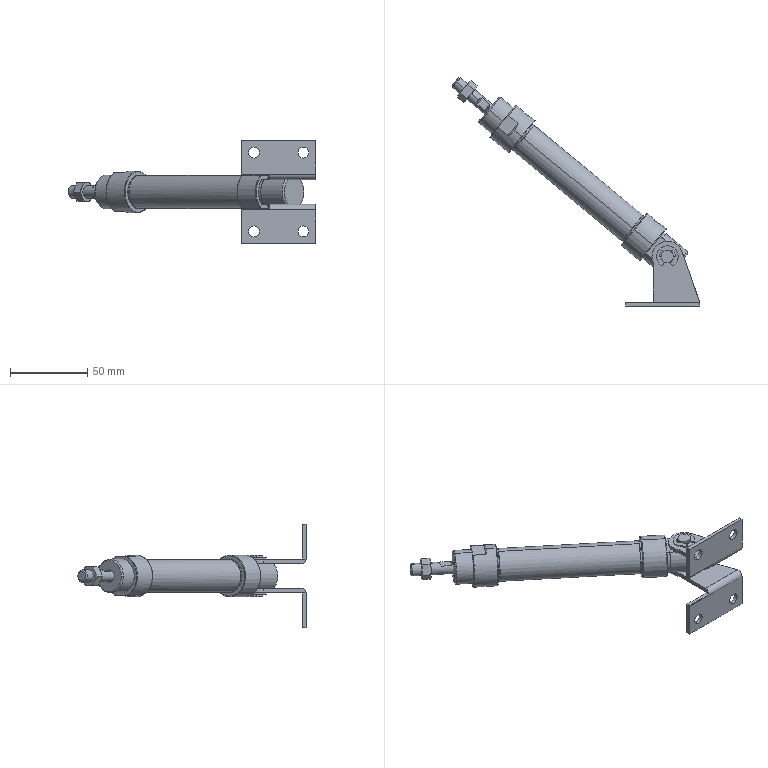Part | SolidWorks | features CompositeCurve 1 | 4 solids | 204 faces | box 160.322 x 147.922 x 67 mm | volume 60763 mm3 | plane 83 | cylinder 82 | cone 31 | spline 8 | commonest cylinder face diameters 8 x16 1 x14 7 x14 14 x6 21.4 x6 8.566 x4